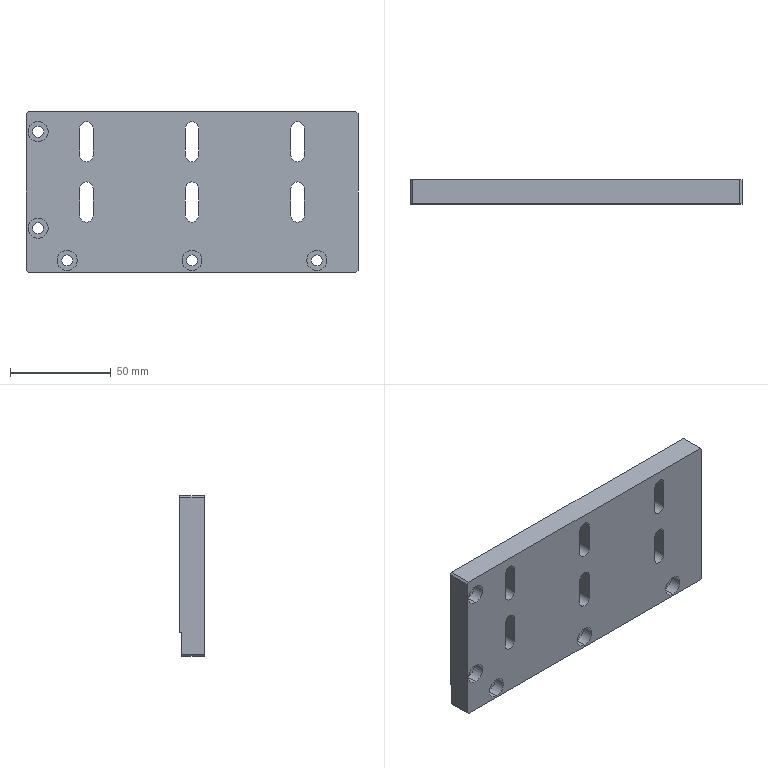Part | SolidWorks | features HoleWzd 3, Chamfer 1, Extrusion 1, ICE 1 | 1 solid | 67 faces | box 165 x 12 x 80 mm | volume 144651 mm3 | cylinder 38 | plane 29 | commonest cylinder face diameters 6.6 x18 5.5 x10 10 x10